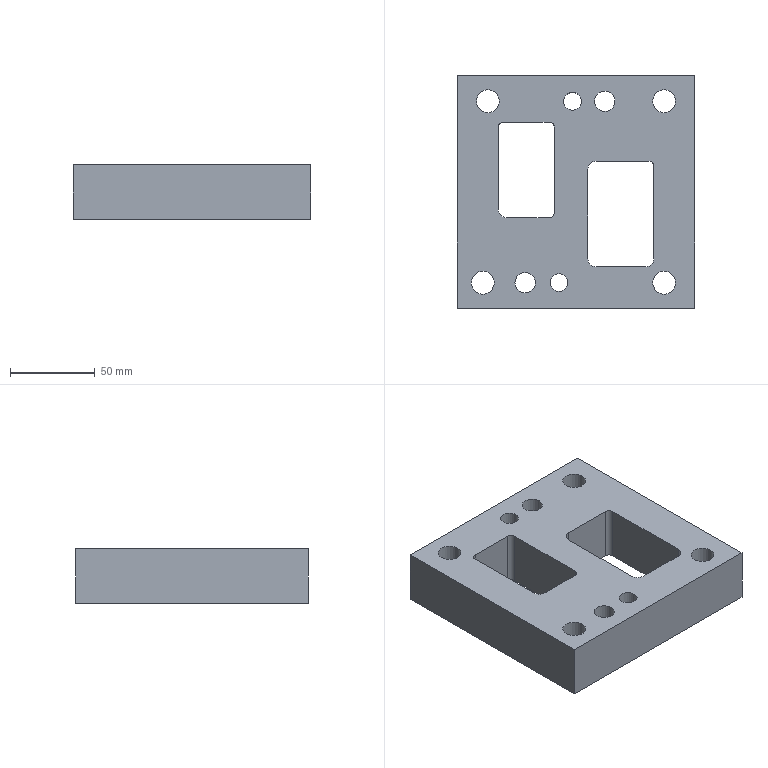Part | STEP file | lll_id3154_x_t | 1 solid | 38 faces | box 140 x 137 x 32 mm | volume 435633 mm3 | cylinder 20 | plane 18 | commonest cylinder face diameters 6 x4 10 x4 13.509 x4 20.008 x4 10.505 x2 12 x2
STEP:
#1=CARTESIAN_POINT('',(469.623,-270.25,60.5));
#2=VERTEX_POINT('',#1);
#3=CARTESIAN_POINT('',(464.37,-270.25,60.5));
#4=DIRECTION('',(0.,0.,1.));
#5=DIRECTION('',(1.,0.,0.));
#6=AXIS2_PLACEMENT_3D('',#3,#4,#5);
#7=CIRCLE('',#6,5.253);
#8=EDGE_CURVE('',#2,#2,#7,.T.);
#9=ORIENTED_EDGE('',*,*,#8,.T.);
#10=EDGE_LOOP('',(#9));
#11=FACE_BOUND('',#10,.T.);
#12=CARTESIAN_POINT('',(528.374,-377.25,60.5));
#13=VERTEX_POINT('',#12);
#14=CARTESIAN_POINT('',(518.37,-377.25,60.5));
#15=DIRECTION('',(0.,0.,-1.));
#16=DIRECTION('',(1.,0.,0.));
#17=AXIS2_PLACEMENT_3D('',#14,#15,#16);
#18=CIRCLE('',#17,10.004);
#19=EDGE_CURVE('',#13,#13,#18,.T.);
#20=ORIENTED_EDGE('',*,*,#19,.F.);
#21=EDGE_LOOP('',(#20));
#22=FACE_BOUND('',#21,.T.);
#23=CARTESIAN_POINT('',(442.371,-377.25,60.5));
#24=VERTEX_POINT('',#23);
#25=CARTESIAN_POINT('',(436.37,-377.25,60.5));
#26=DIRECTION('',(0.,0.,-1.));
#27=DIRECTION('',(1.,0.,0.));
#28=AXIS2_PLACEMENT_3D('',#25,#26,#27);
#29=CIRCLE('',#28,6.);
#30=EDGE_CURVE('',#24,#24,#29,.T.);
#31=ORIENTED_EDGE('',*,*,#30,.F.);
#32=EDGE_LOOP('',(#31));
#33=FACE_BOUND('',#32,.T.);
#34=CARTESIAN_POINT('',(528.374,-270.25,60.5));
#35=VERTEX_POINT('',#34);
#36=CARTESIAN_POINT('',(518.37,-270.25,60.5));
#37=DIRECTION('',(0.,0.,1.));
#38=DIRECTION('',(1.,0.,0.));
#39=AXIS2_PLACEMENT_3D('',#36,#37,#38);
#40=CIRCLE('',#39,10.004);
#41=EDGE_CURVE('',#35,#35,#40,.T.);
#42=ORIENTED_EDGE('',*,*,#41,.T.);
#43=EDGE_LOOP('',(#42));
#44=FACE_BOUND('',#43,.T.);
#45=CARTESIAN_POINT('',(507.37,-368.,60.5));
#46=VERTEX_POINT('',#45);
#47=CARTESIAN_POINT('',(478.37,-368.,60.5));
#48=VERTEX_POINT('',#47);
#49=CARTESIAN_POINT('',(492.87,-368.,60.5));
#50=DIRECTION('',(-1.,0.,0.));
#51=VECTOR('',#50,1.);
#52=LINE('',#49,#51);
#53=EDGE_CURVE('',#46,#48,#52,.T.);
#54=ORIENTED_EDGE('',*,*,#53,.F.);
#55=CARTESIAN_POINT('',(512.37,-363.,60.5));
#56=VERTEX_POINT('',#55);
#57=CARTESIAN_POINT('',(507.37,-363.,60.5));
#58=DIRECTION('',(0.,0.,1.));
#59=DIRECTION('',(-1.,0.,0.));
#60=AXIS2_PLACEMENT_3D('',#57,#58,#59);
#61=CIRCLE('',#60,5.);
#62=EDGE_CURVE('',#46,#56,#61,.T.);
#63=ORIENTED_EDGE('',*,*,#62,.T.);
#64=CARTESIAN_POINT('',(512.37,-308.5,60.5));
#65=VERTEX_POINT('',#64);
#66=CARTESIAN_POINT('',(512.37,-347.5,60.5));
#67=DIRECTION('',(0.,-1.,0.));
#68=VECTOR('',#67,1.);
#69=LINE('',#66,#68);
#70=EDGE_CURVE('',#65,#56,#69,.T.);
#71=ORIENTED_EDGE('',*,*,#70,.F.);
#72=CARTESIAN_POINT('',(509.37,-305.5,60.5));
#73=VERTEX_POINT('',#72);
#74=CARTESIAN_POINT('',(509.37,-308.5,60.5));
#75=DIRECTION('',(0.,0.,1.));
#76=DIRECTION('',(-1.,0.,0.));
#77=AXIS2_PLACEMENT_3D('',#74,#75,#76);
#78=CIRCLE('',#77,3.);
#79=EDGE_CURVE('',#65,#73,#78,.T.);
#80=ORIENTED_EDGE('',*,*,#79,.T.);
#81=CARTESIAN_POINT('',(478.37,-305.5,60.5));
#82=VERTEX_POINT('',#81);
#83=CARTESIAN_POINT('',(492.87,-305.5,60.5));
#84=DIRECTION('',(1.,0.,0.));
#85=VECTOR('',#84,1.);
#86=LINE('',#83,#85);
#87=EDGE_CURVE('',#82,#73,#86,.T.);
#88=ORIENTED_EDGE('',*,*,#87,.F.);
#89=CARTESIAN_POINT('',(473.37,-310.5,60.5));
#90=VERTEX_POINT('',#89);
#91=CARTESIAN_POINT('',(478.37,-310.5,60.5));
#92=DIRECTION('',(0.,0.,1.));
#93=DIRECTION('',(-1.,0.,0.));
#94=AXIS2_PLACEMENT_3D('',#91,#92,#93);
#95=CIRCLE('',#94,5.);
#96=EDGE_CURVE('',#82,#90,#95,.T.);
#97=ORIENTED_EDGE('',*,*,#96,.T.);
#98=CARTESIAN_POINT('',(473.37,-363.,60.5));
#99=VERTEX_POINT('',#98);
#100=CARTESIAN_POINT('',(473.37,-347.5,60.5));
#101=DIRECTION('',(0.,1.,0.));
#102=VECTOR('',#101,1.);
#103=LINE('',#100,#102);
#104=EDGE_CURVE('',#99,#90,#103,.T.);
#105=ORIENTED_EDGE('',*,*,#104,.F.);
#106=CARTESIAN_POINT('',(478.37,-363.,60.5));
#107=DIRECTION('',(0.,0.,1.));
#108=DIRECTION('',(-1.,0.,0.));
#109=AXIS2_PLACEMENT_3D('',#106,#107,#108);
#110=CIRCLE('',#109,5.);
#111=EDGE_CURVE('',#99,#48,#110,.T.);
#112=ORIENTED_EDGE('',*,*,#111,.T.);
#113=EDGE_LOOP('',(#54,#63,#71,#80,#88,#97,#105,#112));
#114=FACE_BOUND('',#113,.T.);
#115=CARTESIAN_POINT('',(536.37,-255.25,60.5));
#116=VERTEX_POINT('',#115);
#117=CARTESIAN_POINT('',(396.37,-255.25,60.5));
#118=VERTEX_POINT('',#117);
#119=CARTESIAN_POINT('',(466.37,-255.25,60.5));
#120=DIRECTION('',(-1.,0.,0.));
#121=VECTOR('',#120,1.);
#122=LINE('',#119,#121);
#123=EDGE_CURVE('',#116,#118,#122,.T.);
#124=ORIENTED_EDGE('',*,*,#123,.F.);
#125=CARTESIAN_POINT('',(536.37,-392.25,60.5));
#126=VERTEX_POINT('',#125);
#127=CARTESIAN_POINT('',(536.37,-325.25,60.5));
#128=DIRECTION('',(0.,1.,0.));
#129=VECTOR('',#128,1.);
#130=LINE('',#127,#129);
#131=EDGE_CURVE('',#126,#116,#130,.T.);
#132=ORIENTED_EDGE('',*,*,#131,.F.);
#133=CARTESIAN_POINT('',(396.37,-392.25,60.5));
#134=VERTEX_POINT('',#133);
#135=CARTESIAN_POINT('',(466.37,-392.25,60.5));
#136=DIRECTION('',(1.,0.,0.));
#137=VECTOR('',#136,1.);
#138=LINE('',#135,#137);
#139=EDGE_CURVE('',#134,#126,#138,.T.);
#140=ORIENTED_EDGE('',*,*,#139,.F.);
#141=CARTESIAN_POINT('',(396.37,-325.25,60.5));
#142=DIRECTION('',(0.,-1.,0.));
#143=VECTOR('',#142,1.);
#144=LINE('',#141,#143);
#145=EDGE_CURVE('',#118,#134,#144,.T.);
#146=ORIENTED_EDGE('',*,*,#145,.F.);
#147=EDGE_LOOP('',(#124,#132,#140,#146));
#148=FACE_BOUND('',#147,.T.);
#149=CARTESIAN_POINT('',(450.5,-282.5,60.5));
#150=VERTEX_POINT('',#149);
#151=CARTESIAN_POINT('',(423.5,-282.5,60.5));
#152=VERTEX_POINT('',#151);
#153=CARTESIAN_POINT('',(437.,-282.5,60.5));
#154=DIRECTION('',(-1.,0.,0.));
#155=VECTOR('',#154,1.);
#156=LINE('',#153,#155);
#157=EDGE_CURVE('',#150,#152,#156,.T.);
#158=ORIENTED_EDGE('',*,*,#157,.T.);
#159=CARTESIAN_POINT('',(420.5,-285.5,60.5));
#160=VERTEX_POINT('',#159);
#161=CARTESIAN_POINT('',(423.5,-285.5,60.5));
#162=DIRECTION('',(0.,0.,1.));
#163=DIRECTION('',(-1.,0.,0.));
#164=AXIS2_PLACEMENT_3D('',#161,#162,#163);
#165=CIRCLE('',#164,3.);
#166=EDGE_CURVE('',#152,#160,#165,.T.);
#167=ORIENTED_EDGE('',*,*,#166,.T.);
#168=CARTESIAN_POINT('',(420.5,-334.,60.5));
#169=VERTEX_POINT('',#168);
#170=CARTESIAN_POINT('',(420.5,-300.,60.5));
#171=DIRECTION('',(0.,-1.,0.));
#172=VECTOR('',#171,1.);
#173=LINE('',#170,#172);
#174=EDGE_CURVE('',#160,#169,#173,.T.);
#175=ORIENTED_EDGE('',*,*,#174,.T.);
#176=CARTESIAN_POINT('',(425.5,-339.,60.5));
#177=VERTEX_POINT('',#176);
#178=CARTESIAN_POINT('',(425.5,-334.,60.5));
#179=DIRECTION('',(0.,0.,1.));
#180=DIRECTION('',(-1.,0.,0.));
#181=AXIS2_PLACEMENT_3D('',#178,#179,#180);
#182=CIRCLE('',#181,5.);
#183=EDGE_CURVE('',#169,#177,#182,.T.);
#184=ORIENTED_EDGE('',*,*,#183,.T.);
#185=CARTESIAN_POINT('',(450.5,-339.,60.5));
#186=VERTEX_POINT('',#185);
#187=CARTESIAN_POINT('',(437.,-339.,60.5));
#188=DIRECTION('',(1.,0.,0.));
#189=VECTOR('',#188,1.);
#190=LINE('',#187,#189);
#191=EDGE_CURVE('',#177,#186,#190,.T.);
#192=ORIENTED_EDGE('',*,*,#191,.T.);
#193=CARTESIAN_POINT('',(453.5,-336.,60.5));
#194=VERTEX_POINT('',#193);
#195=CARTESIAN_POINT('',(450.5,-336.,60.5));
#196=DIRECTION('',(0.,0.,1.));
#197=DIRECTION('',(-1.,0.,0.));
#198=AXIS2_PLACEMENT_3D('',#195,#196,#197);
#199=CIRCLE('',#198,3.);
#200=EDGE_CURVE('',#186,#194,#199,.T.);
#201=ORIENTED_EDGE('',*,*,#200,.T.);
#202=CARTESIAN_POINT('',(453.5,-285.5,60.5));
#203=VERTEX_POINT('',#202);
#204=CARTESIAN_POINT('',(453.5,-300.,60.5));
#205=DIRECTION('',(0.,1.,0.));
#206=VECTOR('',#205,1.);
#207=LINE('',#204,#206);
#208=EDGE_CURVE('',#194,#203,#207,.T.);
#209=ORIENTED_EDGE('',*,*,#208,.T.);
#210=CARTESIAN_POINT('',(450.5,-285.5,60.5));
#211=DIRECTION('',(0.,0.,1.));
#212=DIRECTION('',(-1.,0.,0.));
#213=AXIS2_PLACEMENT_3D('',#210,#211,#212);
#214=CIRCLE('',#213,3.);
#215=EDGE_CURVE('',#203,#150,#214,.T.);
#216=ORIENTED_EDGE('',*,*,#215,.T.);
#217=EDGE_LOOP('',(#158,#167,#175,#184,#192,#201,#209,#216));
#218=FACE_BOUND('',#217,.T.);
#219=CARTESIAN_POINT('',(477.37,-270.25,60.5));
#220=VERTEX_POINT('',#219);
#221=CARTESIAN_POINT('',(483.37,-270.25,60.5));
#222=DIRECTION('',(0.,0.,-1.));
#223=DIRECTION('',(-1.,0.,0.));
#224=AXIS2_PLACEMENT_3D('',#221,#222,#223);
#225=CIRCLE('',#224,6.);
#226=EDGE_CURVE('',#220,#220,#225,.T.);
#227=ORIENTED_EDGE('',*,*,#226,.F.);
#228=EDGE_LOOP('',(#227));
#229=FACE_BOUND('',#228,.T.);
#230=CARTESIAN_POINT('',(404.366,-270.25,60.5));
#231=VERTEX_POINT('',#230);
#232=CARTESIAN_POINT('',(414.37,-270.25,60.5));
#233=DIRECTION('',(0.,0.,-1.));
#234=DIRECTION('',(-1.,0.,0.));
#235=AXIS2_PLACEMENT_3D('',#232,#233,#234);
#236=CIRCLE('',#235,10.004);
#237=EDGE_CURVE('',#231,#231,#236,.T.);
#238=ORIENTED_EDGE('',*,*,#237,.F.);
#239=EDGE_LOOP('',(#238));
#240=FACE_BOUND('',#239,.T.);
#241=CARTESIAN_POINT('',(401.366,-377.25,60.5));
#242=VERTEX_POINT('',#241);
#243=CARTESIAN_POINT('',(411.37,-377.25,60.5));
#244=DIRECTION('',(0.,0.,1.));
#245=DIRECTION('',(-1.,0.,0.));
#246=AXIS2_PLACEMENT_3D('',#243,#244,#245);
#247=CIRCLE('',#246,10.004);
#248=EDGE_CURVE('',#242,#242,#247,.T.);
#249=ORIENTED_EDGE('',*,*,#248,.T.);
#250=EDGE_LOOP('',(#249));
#251=FACE_BOUND('',#250,.T.);
#252=CARTESIAN_POINT('',(461.623,-377.25,60.5));
#253=VERTEX_POINT('',#252);
#254=CARTESIAN_POINT('',(456.37,-377.25,60.5));
#255=DIRECTION('',(0.,0.,1.));
#256=DIRECTION('',(1.,0.,0.));
#257=AXIS2_PLACEMENT_3D('',#254,#255,#256);
#258=CIRCLE('',#257,5.253);
#259=EDGE_CURVE('',#253,#253,#258,.T.);
#260=ORIENTED_EDGE('',*,*,#259,.T.);
#261=EDGE_LOOP('',(#260));
#262=FACE_BOUND('',#261,.T.);
#263=CARTESIAN_POINT('',(466.37,-325.25,60.5));
#264=DIRECTION('',(0.,0.,-1.));
#265=DIRECTION('',(0.,-1.,0.));
#266=AXIS2_PLACEMENT_3D('',#263,#264,#265);
#267=PLANE('',#266);
#268=ADVANCED_FACE('',(#11,#22,#33,#44,#114,#148,#218,#229,#240,#251,#262),#267,.T.);
#269=CARTESIAN_POINT('',(461.623,-377.25,92.5));
#270=VERTEX_POINT('',#269);
#271=CARTESIAN_POINT('',(456.37,-377.25,92.5));
#272=DIRECTION('',(0.,0.,1.));
#273=DIRECTION('',(1.,0.,0.));
#274=AXIS2_PLACEMENT_3D('',#271,#272,#273);
#275=CIRCLE('',#274,5.253);
#276=EDGE_CURVE('',#270,#270,#275,.T.);
#277=ORIENTED_EDGE('',*,*,#276,.F.);
#278=EDGE_LOOP('',(#277));
#279=FACE_BOUND('',#278,.T.);
#280=CARTESIAN_POINT('',(469.623,-270.25,92.5));
#281=VERTEX_POINT('',#280);
#282=CARTESIAN_POINT('',(464.37,-270.25,92.5));
#283=DIRECTION('',(0.,0.,1.));
#284=DIRECTION('',(1.,0.,0.));
#285=AXIS2_PLACEMENT_3D('',#282,#283,#284);
#286=CIRCLE('',#285,5.253);
#287=EDGE_CURVE('',#281,#281,#286,.T.);
#288=ORIENTED_EDGE('',*,*,#287,.F.);
#289=EDGE_LOOP('',(#288));
#290=FACE_BOUND('',#289,.T.);
#291=CARTESIAN_POINT('',(525.125,-377.25,92.5));
#292=VERTEX_POINT('',#291);
#293=CARTESIAN_POINT('',(518.37,-377.25,92.5));
#294=DIRECTION('',(0.,0.,1.));
#295=DIRECTION('',(1.,0.,0.));
#296=AXIS2_PLACEMENT_3D('',#293,#294,#295);
#297=CIRCLE('',#296,6.755);
#298=EDGE_CURVE('',#292,#292,#297,.T.);
#299=ORIENTED_EDGE('',*,*,#298,.F.);
#300=EDGE_LOOP('',(#299));
#301=FACE_BOUND('',#300,.T.);
#302=CARTESIAN_POINT('',(418.125,-377.25,92.5));
#303=VERTEX_POINT('',#302);
#304=CARTESIAN_POINT('',(411.37,-377.25,92.5));
#305=DIRECTION('',(0.,0.,1.));
#306=DIRECTION('',(1.,0.,0.));
#307=AXIS2_PLACEMENT_3D('',#304,#305,#306);
#308=CIRCLE('',#307,6.755);
#309=EDGE_CURVE('',#303,#303,#308,.T.);
#310=ORIENTED_EDGE('',*,*,#309,.F.);
#311=EDGE_LOOP('',(#310));
#312=FACE_BOUND('',#311,.T.);
#313=CARTESIAN_POINT('',(421.125,-270.25,92.5));
#314=VERTEX_POINT('',#313);
#315=CARTESIAN_POINT('',(414.37,-270.25,92.5));
#316=DIRECTION('',(0.,0.,1.));
#317=DIRECTION('',(1.,0.,0.));
#318=AXIS2_PLACEMENT_3D('',#315,#316,#317);
#319=CIRCLE('',#318,6.755);
#320=EDGE_CURVE('',#314,#314,#319,.T.);
#321=ORIENTED_EDGE('',*,*,#320,.F.);
#322=EDGE_LOOP('',(#321));
#323=FACE_BOUND('',#322,.T.);
#324=CARTESIAN_POINT('',(525.125,-270.25,92.5));
#325=VERTEX_POINT('',#324);
#326=CARTESIAN_POINT('',(518.37,-270.25,92.5));
#327=DIRECTION('',(0.,0.,1.));
#328=DIRECTION('',(1.,0.,0.));
#329=AXIS2_PLACEMENT_3D('',#326,#327,#328);
#330=CIRCLE('',#329,6.755);
#331=EDGE_CURVE('',#325,#325,#330,.T.);
#332=ORIENTED_EDGE('',*,*,#331,.F.);
#333=EDGE_LOOP('',(#332));
#334=FACE_BOUND('',#333,.T.);
#335=CARTESIAN_POINT('',(536.37,-255.25,92.5));
#336=VERTEX_POINT('',#335);
#337=CARTESIAN_POINT('',(536.37,-392.25,92.5));
#338=VERTEX_POINT('',#337);
#339=CARTESIAN_POINT('',(536.37,-325.25,92.5));
#340=DIRECTION('',(0.,-1.,0.));
#341=VECTOR('',#340,1.);
#342=LINE('',#339,#341);
#343=EDGE_CURVE('',#336,#338,#342,.T.);
#344=ORIENTED_EDGE('',*,*,#343,.F.);
#345=CARTESIAN_POINT('',(396.37,-255.25,92.5));
#346=VERTEX_POINT('',#345);
#347=CARTESIAN_POINT('',(466.37,-255.25,92.5));
#348=DIRECTION('',(1.,0.,0.));
#349=VECTOR('',#348,1.);
#350=LINE('',#347,#349);
#351=EDGE_CURVE('',#346,#336,#350,.T.);
#352=ORIENTED_EDGE('',*,*,#351,.F.);
#353=CARTESIAN_POINT('',(396.37,-392.25,92.5));
#354=VERTEX_POINT('',#353);
#355=CARTESIAN_POINT('',(396.37,-325.25,92.5));
#356=DIRECTION('',(0.,1.,0.));
#357=VECTOR('',#356,1.);
#358=LINE('',#355,#357);
#359=EDGE_CURVE('',#354,#346,#358,.T.);
#360=ORIENTED_EDGE('',*,*,#359,.F.);
#361=CARTESIAN_POINT('',(466.37,-392.25,92.5));
#362=DIRECTION('',(-1.,0.,0.));
#363=VECTOR('',#362,1.);
#364=LINE('',#361,#363);
#365=EDGE_CURVE('',#338,#354,#364,.T.);
#366=ORIENTED_EDGE('',*,*,#365,.F.);
#367=EDGE_LOOP('',(#344,#352,#360,#366));
#368=FACE_BOUND('',#367,.T.);
#369=CARTESIAN_POINT('',(509.37,-305.5,92.5));
#370=VERTEX_POINT('',#369);
#371=CARTESIAN_POINT('',(478.37,-305.5,92.5));
#372=VERTEX_POINT('',#371);
#373=CARTESIAN_POINT('',(492.87,-305.5,92.5));
#374=DIRECTION('',(-1.,0.,0.));
#375=VECTOR('',#374,1.);
#376=LINE('',#373,#375);
#377=EDGE_CURVE('',#370,#372,#376,.T.);
#378=ORIENTED_EDGE('',*,*,#377,.F.);
#379=CARTESIAN_POINT('',(512.37,-308.5,92.5));
#380=VERTEX_POINT('',#379);
#381=CARTESIAN_POINT('',(509.37,-308.5,92.5));
#382=DIRECTION('',(0.,0.,-1.));
#383=DIRECTION('',(1.,0.,0.));
#384=AXIS2_PLACEMENT_3D('',#381,#382,#383);
#385=CIRCLE('',#384,3.);
#386=EDGE_CURVE('',#370,#380,#385,.T.);
#387=ORIENTED_EDGE('',*,*,#386,.T.);
#388=CARTESIAN_POINT('',(512.37,-363.,92.5));
#389=VERTEX_POINT('',#388);
#390=CARTESIAN_POINT('',(512.37,-347.5,92.5));
#391=DIRECTION('',(0.,1.,0.));
#392=VECTOR('',#391,1.);
#393=LINE('',#390,#392);
#394=EDGE_CURVE('',#389,#380,#393,.T.);
#395=ORIENTED_EDGE('',*,*,#394,.F.);
#396=CARTESIAN_POINT('',(507.37,-368.,92.5));
#397=VERTEX_POINT('',#396);
#398=CARTESIAN_POINT('',(507.37,-363.,92.5));
#399=DIRECTION('',(0.,0.,-1.));
#400=DIRECTION('',(1.,0.,0.));
#401=AXIS2_PLACEMENT_3D('',#398,#399,#400);
#402=CIRCLE('',#401,5.);
#403=EDGE_CURVE('',#389,#397,#402,.T.);
#404=ORIENTED_EDGE('',*,*,#403,.T.);
#405=CARTESIAN_POINT('',(478.37,-368.,92.5));
#406=VERTEX_POINT('',#405);
#407=CARTESIAN_POINT('',(492.87,-368.,92.5));
#408=DIRECTION('',(1.,0.,0.));
#409=VECTOR('',#408,1.);
#410=LINE('',#407,#409);
#411=EDGE_CURVE('',#406,#397,#410,.T.);
#412=ORIENTED_EDGE('',*,*,#411,.F.);
#413=CARTESIAN_POINT('',(473.37,-363.,92.5));
#414=VERTEX_POINT('',#413);
#415=CARTESIAN_POINT('',(478.37,-363.,92.5));
#416=DIRECTION('',(0.,0.,-1.));
#417=DIRECTION('',(1.,0.,0.));
#418=AXIS2_PLACEMENT_3D('',#415,#416,#417);
#419=CIRCLE('',#418,5.);
#420=EDGE_CURVE('',#406,#414,#419,.T.);
#421=ORIENTED_EDGE('',*,*,#420,.T.);
#422=CARTESIAN_POINT('',(473.37,-310.5,92.5));
#423=VERTEX_POINT('',#422);
#424=CARTESIAN_POINT('',(473.37,-347.5,92.5));
#425=DIRECTION('',(0.,-1.,0.));
#426=VECTOR('',#425,1.);
#427=LINE('',#424,#426);
#428=EDGE_CURVE('',#423,#414,#427,.T.);
#429=ORIENTED_EDGE('',*,*,#428,.F.);
#430=CARTESIAN_POINT('',(478.37,-310.5,92.5));
#431=DIRECTION('',(0.,0.,-1.));
#432=DIRECTION('',(1.,0.,0.));
#433=AXIS2_PLACEMENT_3D('',#430,#431,#432);
#434=CIRCLE('',#433,5.);
#435=EDGE_CURVE('',#423,#372,#434,.T.);
#436=ORIENTED_EDGE('',*,*,#435,.T.);
#437=EDGE_LOOP('',(#378,#387,#395,#404,#412,#421,#429,#436));
#438=FACE_BOUND('',#437,.T.);
#439=CARTESIAN_POINT('',(420.5,-334.,92.5));
#440=VERTEX_POINT('',#439);
#441=CARTESIAN_POINT('',(420.5,-285.5,92.5));
#442=VERTEX_POINT('',#441);
#443=CARTESIAN_POINT('',(420.5,-300.,92.5));
#444=DIRECTION('',(0.,1.,0.));
#445=VECTOR('',#444,1.);
#446=LINE('',#443,#445);
#447=EDGE_CURVE('',#440,#442,#446,.T.);
#448=ORIENTED_EDGE('',*,*,#447,.T.);
#449=CARTESIAN_POINT('',(423.5,-282.5,92.5));
#450=VERTEX_POINT('',#449);
#451=CARTESIAN_POINT('',(423.5,-285.5,92.5));
#452=DIRECTION('',(0.,0.,-1.));
#453=DIRECTION('',(1.,0.,0.));
#454=AXIS2_PLACEMENT_3D('',#451,#452,#453);
#455=CIRCLE('',#454,3.);
#456=EDGE_CURVE('',#442,#450,#455,.T.);
#457=ORIENTED_EDGE('',*,*,#456,.T.);
#458=CARTESIAN_POINT('',(450.5,-282.5,92.5));
#459=VERTEX_POINT('',#458);
#460=CARTESIAN_POINT('',(437.,-282.5,92.5));
#461=DIRECTION('',(1.,0.,0.));
#462=VECTOR('',#461,1.);
#463=LINE('',#460,#462);
#464=EDGE_CURVE('',#450,#459,#463,.T.);
#465=ORIENTED_EDGE('',*,*,#464,.T.);
#466=CARTESIAN_POINT('',(453.5,-285.5,92.5));
#467=VERTEX_POINT('',#466);
#468=CARTESIAN_POINT('',(450.5,-285.5,92.5));
#469=DIRECTION('',(0.,0.,-1.));
#470=DIRECTION('',(1.,0.,0.));
#471=AXIS2_PLACEMENT_3D('',#468,#469,#470);
#472=CIRCLE('',#471,3.);
#473=EDGE_CURVE('',#459,#467,#472,.T.);
#474=ORIENTED_EDGE('',*,*,#473,.T.);
#475=CARTESIAN_POINT('',(453.5,-336.,92.5));
#476=VERTEX_POINT('',#475);
#477=CARTESIAN_POINT('',(453.5,-300.,92.5));
#478=DIRECTION('',(0.,-1.,0.));
#479=VECTOR('',#478,1.);
#480=LINE('',#477,#479);
#481=EDGE_CURVE('',#467,#476,#480,.T.);
#482=ORIENTED_EDGE('',*,*,#481,.T.);
#483=CARTESIAN_POINT('',(450.5,-339.,92.5));
#484=VERTEX_POINT('',#483);
#485=CARTESIAN_POINT('',(450.5,-336.,92.5));
#486=DIRECTION('',(0.,0.,-1.));
#487=DIRECTION('',(1.,0.,0.));
#488=AXIS2_PLACEMENT_3D('',#485,#486,#487);
#489=CIRCLE('',#488,3.);
#490=EDGE_CURVE('',#476,#484,#489,.T.);
#491=ORIENTED_EDGE('',*,*,#490,.T.);
#492=CARTESIAN_POINT('',(425.5,-339.,92.5));
#493=VERTEX_POINT('',#492);
#494=CARTESIAN_POINT('',(437.,-339.,92.5));
#495=DIRECTION('',(-1.,0.,0.));
#496=VECTOR('',#495,1.);
#497=LINE('',#494,#496);
#498=EDGE_CURVE('',#484,#493,#497,.T.);
#499=ORIENTED_EDGE('',*,*,#498,.T.);
#500=CARTESIAN_POINT('',(425.5,-334.,92.5));
#501=DIRECTION('',(0.,0.,-1.));
#502=DIRECTION('',(1.,0.,0.));
#503=AXIS2_PLACEMENT_3D('',#500,#501,#502);
#504=CIRCLE('',#503,5.);
#505=EDGE_CURVE('',#493,#440,#504,.T.);
#506=ORIENTED_EDGE('',*,*,#505,.T.);
#507=EDGE_LOOP('',(#448,#457,#465,#474,#482,#491,#499,#506));
#508=FACE_BOUND('',#507,.T.);
#509=CARTESIAN_POINT('',(489.371,-270.25,92.5));
#510=VERTEX_POINT('',#509);
#511=CARTESIAN_POINT('',(483.37,-270.25,92.5));
#512=DIRECTION('',(0.,0.,-1.));
#513=DIRECTION('',(1.,0.,0.));
#514=AXIS2_PLACEMENT_3D('',#511,#512,#513);
#515=CIRCLE('',#514,6.);
#516=EDGE_CURVE('',#510,#510,#515,.T.);
#517=ORIENTED_EDGE('',*,*,#516,.T.);
#518=EDGE_LOOP('',(#517));
#519=FACE_BOUND('',#518,.T.);
#520=CARTESIAN_POINT('',(430.37,-377.25,92.5));
#521=VERTEX_POINT('',#520);
#522=CARTESIAN_POINT('',(436.37,-377.25,92.5));
#523=DIRECTION('',(0.,0.,-1.));
#524=DIRECTION('',(-1.,0.,0.));
#525=AXIS2_PLACEMENT_3D('',#522,#523,#524);
#526=CIRCLE('',#525,6.);
#527=EDGE_CURVE('',#521,#521,#526,.T.);
#528=ORIENTED_EDGE('',*,*,#527,.T.);
#529=EDGE_LOOP('',(#528));
#530=FACE_BOUND('',#529,.T.);
#531=CARTESIAN_POINT('',(466.37,-325.25,92.5));
#532=DIRECTION('',(0.,0.,1.));
#533=DIRECTION('',(0.,1.,0.));
#534=AXIS2_PLACEMENT_3D('',#531,#532,#533);
#535=PLANE('',#534);
#536=ADVANCED_FACE('',(#279,#290,#301,#312,#323,#334,#368,#438,#508,#519,#530),#535,.T.);
#537=CARTESIAN_POINT('',(536.37,-255.25,60.5));
#538=DIRECTION('',(0.,0.,1.));
#539=VECTOR('',#538,1.);
#540=LINE('',#537,#539);
#541=EDGE_CURVE('',#116,#336,#540,.T.);
#542=ORIENTED_EDGE('',*,*,#541,.T.);
#543=ORIENTED_EDGE('',*,*,#343,.T.);
#544=CARTESIAN_POINT('',(536.37,-392.25,60.5));
#545=DIRECTION('',(0.,0.,1.));
#546=VECTOR('',#545,1.);
#547=LINE('',#544,#546);
#548=EDGE_CURVE('',#126,#338,#547,.T.);
#549=ORIENTED_EDGE('',*,*,#548,.F.);
#550=ORIENTED_EDGE('',*,*,#131,.T.);
#551=EDGE_LOOP('',(#542,#543,#549,#550));
#552=FACE_OUTER_BOUND('',#551,.T.);
#553=CARTESIAN_POINT('',(536.37,-325.25,60.5));
#554=DIRECTION('',(1.,0.,0.));
#555=DIRECTION('',(0.,0.,-1.));
#556=AXIS2_PLACEMENT_3D('',#553,#554,#555);
#557=PLANE('',#556);
#558=ADVANCED_FACE('',(#552),#557,.T.);
#559=ORIENTED_EDGE('',*,*,#548,.T.);
#560=ORIENTED_EDGE('',*,*,#365,.T.);
#561=CARTESIAN_POINT('',(396.37,-392.25,60.5));
#562=DIRECTION('',(0.,0.,1.));
#563=VECTOR('',#562,1.);
#564=LINE('',#561,#563);
#565=EDGE_CURVE('',#134,#354,#564,.T.);
#566=ORIENTED_EDGE('',*,*,#565,.F.);
#567=ORIENTED_EDGE('',*,*,#139,.T.);
#568=EDGE_LOOP('',(#559,#560,#566,#567));
#569=FACE_OUTER_BOUND('',#568,.T.);
#570=CARTESIAN_POINT('',(466.37,-392.25,60.5));
#571=DIRECTION('',(0.,-1.,0.));
#572=DIRECTION('',(0.,0.,1.));
#573=AXIS2_PLACEMENT_3D('',#570,#571,#572);
#574=PLANE('',#573);
#575=ADVANCED_FACE('',(#569),#574,.T.);
#576=ORIENTED_EDGE('',*,*,#565,.T.);
#577=ORIENTED_EDGE('',*,*,#359,.T.);
#578=CARTESIAN_POINT('',(396.37,-255.25,60.5));
#579=DIRECTION('',(0.,0.,1.));
#580=VECTOR('',#579,1.);
#581=LINE('',#578,#580);
#582=EDGE_CURVE('',#118,#346,#581,.T.);
#583=ORIENTED_EDGE('',*,*,#582,.F.);
#584=ORIENTED_EDGE('',*,*,#145,.T.);
#585=EDGE_LOOP('',(#576,#577,#583,#584));
#586=FACE_OUTER_BOUND('',#585,.T.);
#587=CARTESIAN_POINT('',(396.37,-325.25,60.5));
#588=DIRECTION('',(-1.,0.,0.));
#589=DIRECTION('',(0.,0.,1.));
#590=AXIS2_PLACEMENT_3D('',#587,#588,#589);
#591=PLANE('',#590);
#592=ADVANCED_FACE('',(#586),#591,.T.);
#593=ORIENTED_EDGE('',*,*,#123,.T.);
#594=ORIENTED_EDGE('',*,*,#582,.T.);
#595=ORIENTED_EDGE('',*,*,#351,.T.);
#596=ORIENTED_EDGE('',*,*,#541,.F.);
#597=EDGE_LOOP('',(#593,#594,#595,#596));
#598=FACE_OUTER_BOUND('',#597,.T.);
#599=CARTESIAN_POINT('',(466.37,-255.25,60.5));
#600=DIRECTION('',(0.,1.,0.));
#601=DIRECTION('',(0.,0.,-1.));
#602=AXIS2_PLACEMENT_3D('',#599,#600,#601);
#603=PLANE('',#602);
#604=ADVANCED_FACE('',(#598),#603,.T.);
#605=ORIENTED_EDGE('',*,*,#411,.T.);
#606=CARTESIAN_POINT('',(507.37,-368.,60.5));
#607=DIRECTION('',(0.,0.,-1.));
#608=VECTOR('',#607,1.);
#609=LINE('',#606,#608);
#610=EDGE_CURVE('',#397,#46,#609,.T.);
#611=ORIENTED_EDGE('',*,*,#610,.T.);
#612=ORIENTED_EDGE('',*,*,#53,.T.);
#613=CARTESIAN_POINT('',(478.37,-368.,92.5));
#614=DIRECTION('',(0.,0.,1.));
#615=VECTOR('',#614,1.);
#616=LINE('',#613,#615);
#617=EDGE_CURVE('',#48,#406,#616,.T.);
#618=ORIENTED_EDGE('',*,*,#617,.T.);
#619=EDGE_LOOP('',(#605,#611,#612,#618));
#620=FACE_OUTER_BOUND('',#619,.T.);
#621=CARTESIAN_POINT('',(492.87,-368.,-8.5));
#622=DIRECTION('',(0.,-1.,0.));
#623=DIRECTION('',(0.,0.,-1.));
#624=AXIS2_PLACEMENT_3D('',#621,#622,#623);
#625=PLANE('',#624);
#626=ADVANCED_FACE('',(#620),#625,.F.);
#627=ORIENTED_EDGE('',*,*,#104,.T.);
#628=CARTESIAN_POINT('',(473.37,-310.5,92.5));
#629=DIRECTION('',(0.,0.,1.));
#630=VECTOR('',#629,1.);
#631=LINE('',#628,#630);
#632=EDGE_CURVE('',#90,#423,#631,.T.);
#633=ORIENTED_EDGE('',*,*,#632,.T.);
#634=ORIENTED_EDGE('',*,*,#428,.T.);
#635=CARTESIAN_POINT('',(473.37,-363.,60.5));
#636=DIRECTION('',(0.,0.,-1.));
#637=VECTOR('',#636,1.);
#638=LINE('',#635,#637);
#639=EDGE_CURVE('',#414,#99,#638,.T.);
#640=ORIENTED_EDGE('',*,*,#639,.T.);
#641=EDGE_LOOP('',(#627,#633,#634,#640));
#642=FACE_OUTER_BOUND('',#641,.T.);
#643=CARTESIAN_POINT('',(473.37,-347.5,-8.5));
#644=DIRECTION('',(-1.,0.,0.));
#645=DIRECTION('',(0.,0.,-1.));
#646=AXIS2_PLACEMENT_3D('',#643,#644,#645);
#647=PLANE('',#646);
#648=ADVANCED_FACE('',(#642),#647,.F.);
#649=ORIENTED_EDGE('',*,*,#87,.T.);
#650=CARTESIAN_POINT('',(509.37,-305.5,92.5));
#651=DIRECTION('',(0.,0.,1.));
#652=VECTOR('',#651,1.);
#653=LINE('',#650,#652);
#654=EDGE_CURVE('',#73,#370,#653,.T.);
#655=ORIENTED_EDGE('',*,*,#654,.T.);
#656=ORIENTED_EDGE('',*,*,#377,.T.);
#657=CARTESIAN_POINT('',(478.37,-305.5,60.5));
#658=DIRECTION('',(0.,0.,-1.));
#659=VECTOR('',#658,1.);
#660=LINE('',#657,#659);
#661=EDGE_CURVE('',#372,#82,#660,.T.);
#662=ORIENTED_EDGE('',*,*,#661,.T.);
#663=EDGE_LOOP('',(#649,#655,#656,#662));
#664=FACE_OUTER_BOUND('',#663,.T.);
#665=CARTESIAN_POINT('',(492.87,-305.5,-8.5));
#666=DIRECTION('',(0.,1.,0.));
#667=DIRECTION('',(0.,0.,1.));
#668=AXIS2_PLACEMENT_3D('',#665,#666,#667);
#669=PLANE('',#668);
#670=ADVANCED_FACE('',(#664),#669,.F.);
#671=ORIENTED_EDGE('',*,*,#394,.T.);
#672=CARTESIAN_POINT('',(512.37,-308.5,60.5));
#673=DIRECTION('',(0.,0.,-1.));
#674=VECTOR('',#673,1.);
#675=LINE('',#672,#674);
#676=EDGE_CURVE('',#380,#65,#675,.T.);
#677=ORIENTED_EDGE('',*,*,#676,.T.);
#678=ORIENTED_EDGE('',*,*,#70,.T.);
#679=CARTESIAN_POINT('',(512.37,-363.,92.5));
#680=DIRECTION('',(0.,0.,1.));
#681=VECTOR('',#680,1.);
#682=LINE('',#679,#681);
#683=EDGE_CURVE('',#56,#389,#682,.T.);
#684=ORIENTED_EDGE('',*,*,#683,.T.);
#685=EDGE_LOOP('',(#671,#677,#678,#684));
#686=FACE_OUTER_BOUND('',#685,.T.);
#687=CARTESIAN_POINT('',(512.37,-347.5,-8.5));
#688=DIRECTION('',(1.,0.,0.));
#689=DIRECTION('',(0.,0.,1.));
#690=AXIS2_PLACEMENT_3D('',#687,#688,#689);
#691=PLANE('',#690);
#692=ADVANCED_FACE('',(#686),#691,.F.);
#693=ORIENTED_EDGE('',*,*,#498,.F.);
#694=CARTESIAN_POINT('',(450.5,-339.,60.5));
#695=DIRECTION('',(0.,0.,-1.));
#696=VECTOR('',#695,1.);
#697=LINE('',#694,#696);
#698=EDGE_CURVE('',#484,#186,#697,.T.);
#699=ORIENTED_EDGE('',*,*,#698,.T.);
#700=ORIENTED_EDGE('',*,*,#191,.F.);
#701=CARTESIAN_POINT('',(425.5,-339.,92.5));
#702=DIRECTION('',(0.,0.,1.));
#703=VECTOR('',#702,1.);
#704=LINE('',#701,#703);
#705=EDGE_CURVE('',#177,#493,#704,.T.);
#706=ORIENTED_EDGE('',*,*,#705,.T.);
#707=EDGE_LOOP('',(#693,#699,#700,#706));
#708=FACE_OUTER_BOUND('',#707,.T.);
#709=CARTESIAN_POINT('',(437.,-339.,-8.5));
#710=DIRECTION('',(0.,-1.,0.));
#711=DIRECTION('',(0.,0.,1.));
#712=AXIS2_PLACEMENT_3D('',#709,#710,#711);
#713=PLANE('',#712);
#714=ADVANCED_FACE('',(#708),#713,.F.);
#715=ORIENTED_EDGE('',*,*,#174,.F.);
#716=CARTESIAN_POINT('',(420.5,-285.5,92.5));
#717=DIRECTION('',(0.,0.,1.));
#718=VECTOR('',#717,1.);
#719=LINE('',#716,#718);
#720=EDGE_CURVE('',#160,#442,#719,.T.);
#721=ORIENTED_EDGE('',*,*,#720,.T.);
#722=ORIENTED_EDGE('',*,*,#447,.F.);
#723=CARTESIAN_POINT('',(420.5,-334.,60.5));
#724=DIRECTION('',(0.,0.,-1.));
#725=VECTOR('',#724,1.);
#726=LINE('',#723,#725);
#727=EDGE_CURVE('',#440,#169,#726,.T.);
#728=ORIENTED_EDGE('',*,*,#727,.T.);
#729=EDGE_LOOP('',(#715,#721,#722,#728));
#730=FACE_OUTER_BOUND('',#729,.T.);
#731=CARTESIAN_POINT('',(420.5,-300.,-8.5));
#732=DIRECTION('',(-1.,0.,0.));
#733=DIRECTION('',(0.,0.,-1.));
#734=AXIS2_PLACEMENT_3D('',#731,#732,#733);
#735=PLANE('',#734);
#736=ADVANCED_FACE('',(#730),#735,.F.);
#737=ORIENTED_EDGE('',*,*,#464,.F.);
#738=CARTESIAN_POINT('',(423.5,-282.5,60.5));
#739=DIRECTION('',(0.,0.,-1.));
#740=VECTOR('',#739,1.);
#741=LINE('',#738,#740);
#742=EDGE_CURVE('',#450,#152,#741,.T.);
#743=ORIENTED_EDGE('',*,*,#742,.T.);
#744=ORIENTED_EDGE('',*,*,#157,.F.);
#745=CARTESIAN_POINT('',(450.5,-282.5,92.5));
#746=DIRECTION('',(0.,0.,1.));
#747=VECTOR('',#746,1.);
#748=LINE('',#745,#747);
#749=EDGE_CURVE('',#150,#459,#748,.T.);
#750=ORIENTED_EDGE('',*,*,#749,.T.);
#751=EDGE_LOOP('',(#737,#743,#744,#750));
#752=FACE_OUTER_BOUND('',#751,.T.);
#753=CARTESIAN_POINT('',(437.,-282.5,-8.5));
#754=DIRECTION('',(0.,1.,0.));
#755=DIRECTION('',(0.,0.,-1.));
#756=AXIS2_PLACEMENT_3D('',#753,#754,#755);
#757=PLANE('',#756);
#758=ADVANCED_FACE('',(#752),#757,.F.);
#759=ORIENTED_EDGE('',*,*,#208,.F.);
#760=CARTESIAN_POINT('',(453.5,-336.,92.5));
#761=DIRECTION('',(0.,0.,1.));
#762=VECTOR('',#761,1.);
#763=LINE('',#760,#762);
#764=EDGE_CURVE('',#194,#476,#763,.T.);
#765=ORIENTED_EDGE('',*,*,#764,.T.);
#766=ORIENTED_EDGE('',*,*,#481,.F.);
#767=CARTESIAN_POINT('',(453.5,-285.5,60.5));
#768=DIRECTION('',(0.,0.,-1.));
#769=VECTOR('',#768,1.);
#770=LINE('',#767,#769);
#771=EDGE_CURVE('',#467,#203,#770,.T.);
#772=ORIENTED_EDGE('',*,*,#771,.T.);
#773=EDGE_LOOP('',(#759,#765,#766,#772));
#774=FACE_OUTER_BOUND('',#773,.T.);
#775=CARTESIAN_POINT('',(453.5,-300.,-8.5));
#776=DIRECTION('',(1.,0.,0.));
#777=DIRECTION('',(0.,0.,1.));
#778=AXIS2_PLACEMENT_3D('',#775,#776,#777);
#779=PLANE('',#778);
#780=ADVANCED_FACE('',(#774),#779,.F.);
#781=CARTESIAN_POINT('',(528.374,-270.25,75.5));
#782=VERTEX_POINT('',#781);
#783=CARTESIAN_POINT('',(518.37,-270.25,75.5));
#784=DIRECTION('',(0.,0.,1.));
#785=DIRECTION('',(1.,0.,0.));
#786=AXIS2_PLACEMENT_3D('',#783,#784,#785);
#787=CIRCLE('',#786,10.004);
#788=EDGE_CURVE('',#782,#782,#787,.T.);
#789=ORIENTED_EDGE('',*,*,#788,.T.);
#790=EDGE_LOOP('',(#789));
#791=FACE_BOUND('',#790,.T.);
#792=ORIENTED_EDGE('',*,*,#41,.F.);
#793=EDGE_LOOP('',(#792));
#794=FACE_BOUND('',#793,.T.);
#795=CARTESIAN_POINT('',(518.37,-270.25,60.5));
#796=DIRECTION('',(0.,0.,1.));
#797=DIRECTION('',(1.,0.,0.));
#798=AXIS2_PLACEMENT_3D('',#795,#796,#797);
#799=CYLINDRICAL_SURFACE('',#798,10.004);
#800=ADVANCED_FACE('',(#791,#794),#799,.F.);
#801=ORIENTED_EDGE('',*,*,#331,.T.);
#802=EDGE_LOOP('',(#801));
#803=FACE_BOUND('',#802,.T.);
#804=CARTESIAN_POINT('',(525.125,-270.25,75.5));
#805=VERTEX_POINT('',#804);
#806=CARTESIAN_POINT('',(518.37,-270.25,75.5));
#807=DIRECTION('',(0.,0.,1.));
#808=DIRECTION('',(1.,0.,0.));
#809=AXIS2_PLACEMENT_3D('',#806,#807,#808);
#810=CIRCLE('',#809,6.755);
#811=EDGE_CURVE('',#805,#805,#810,.T.);
#812=ORIENTED_EDGE('',*,*,#811,.F.);
#813=EDGE_LOOP('',(#812));
#814=FACE_BOUND('',#813,.T.);
#815=CARTESIAN_POINT('',(518.37,-270.25,57.5));
#816=DIRECTION('',(0.,0.,1.));
#817=DIRECTION('',(1.,0.,0.));
#818=AXIS2_PLACEMENT_3D('',#815,#816,#817);
#819=CYLINDRICAL_SURFACE('',#818,6.755);
#820=ADVANCED_FACE('',(#803,#814),#819,.F.);
#821=ORIENTED_EDGE('',*,*,#811,.T.);
#822=EDGE_LOOP('',(#821));
#823=FACE_BOUND('',#822,.T.);
#824=ORIENTED_EDGE('',*,*,#788,.F.);
#825=EDGE_LOOP('',(#824));
#826=FACE_BOUND('',#825,.T.);
#827=CARTESIAN_POINT('',(518.37,-270.25,75.5));
#828=DIRECTION('',(0.,0.,1.));
#829=DIRECTION('',(1.,0.,0.));
#830=AXIS2_PLACEMENT_3D('',#827,#828,#829);
#831=PLANE('',#830);
#832=ADVANCED_FACE('',(#823,#826),#831,.F.);
#833=ORIENTED_EDGE('',*,*,#226,.T.);
#834=EDGE_LOOP('',(#833));
#835=FACE_BOUND('',#834,.T.);
#836=ORIENTED_EDGE('',*,*,#516,.F.);
#837=EDGE_LOOP('',(#836));
#838=FACE_BOUND('',#837,.T.);
#839=CARTESIAN_POINT('',(483.37,-270.25,57.5));
#840=DIRECTION('',(0.,0.,1.));
#841=DIRECTION('',(1.,0.,0.));
#842=AXIS2_PLACEMENT_3D('',#839,#840,#841);
#843=CYLINDRICAL_SURFACE('',#842,6.);
#844=ADVANCED_FACE('',(#835,#838),#843,.F.);
#845=CARTESIAN_POINT('',(404.366,-270.25,75.5));
#846=VERTEX_POINT('',#845);
#847=CARTESIAN_POINT('',(414.37,-270.25,75.5));
#848=DIRECTION('',(0.,0.,-1.));
#849=DIRECTION('',(-1.,0.,0.));
#850=AXIS2_PLACEMENT_3D('',#847,#848,#849);
#851=CIRCLE('',#850,10.004);
#852=EDGE_CURVE('',#846,#846,#851,.T.);
#853=ORIENTED_EDGE('',*,*,#852,.F.);
#854=EDGE_LOOP('',(#853));
#855=FACE_BOUND('',#854,.T.);
#856=ORIENTED_EDGE('',*,*,#237,.T.);
#857=EDGE_LOOP('',(#856));
#858=FACE_BOUND('',#857,.T.);
#859=CARTESIAN_POINT('',(414.37,-270.25,60.5));
#860=DIRECTION('',(0.,0.,1.));
#861=DIRECTION('',(-1.,0.,0.));
#862=AXIS2_PLACEMENT_3D('',#859,#860,#861);
#863=CYLINDRICAL_SURFACE('',#862,10.004);
#864=ADVANCED_FACE('',(#855,#858),#863,.F.);
#865=ORIENTED_EDGE('',*,*,#320,.T.);
#866=EDGE_LOOP('',(#865));
#867=FACE_BOUND('',#866,.T.);
#868=CARTESIAN_POINT('',(407.616,-270.25,75.5));
#869=VERTEX_POINT('',#868);
#870=CARTESIAN_POINT('',(414.37,-270.25,75.5));
#871=DIRECTION('',(0.,0.,-1.));
#872=DIRECTION('',(-1.,0.,0.));
#873=AXIS2_PLACEMENT_3D('',#870,#871,#872);
#874=CIRCLE('',#873,6.755);
#875=EDGE_CURVE('',#869,#869,#874,.T.);
#876=ORIENTED_EDGE('',*,*,#875,.T.);
#877=EDGE_LOOP('',(#876));
#878=FACE_BOUND('',#877,.T.);
#879=CARTESIAN_POINT('',(414.37,-270.25,57.5));
#880=DIRECTION('',(0.,0.,1.));
#881=DIRECTION('',(-1.,0.,0.));
#882=AXIS2_PLACEMENT_3D('',#879,#880,#881);
#883=CYLINDRICAL_SURFACE('',#882,6.755);
#884=ADVANCED_FACE('',(#867,#878),#883,.F.);
#885=ORIENTED_EDGE('',*,*,#875,.F.);
#886=EDGE_LOOP('',(#885));
#887=FACE_BOUND('',#886,.T.);
#888=ORIENTED_EDGE('',*,*,#852,.T.);
#889=EDGE_LOOP('',(#888));
#890=FACE_BOUND('',#889,.T.);
#891=CARTESIAN_POINT('',(414.37,-270.25,75.5));
#892=DIRECTION('',(0.,0.,1.));
#893=DIRECTION('',(-1.,0.,0.));
#894=AXIS2_PLACEMENT_3D('',#891,#892,#893);
#895=PLANE('',#894);
#896=ADVANCED_FACE('',(#887,#890),#895,.F.);
#897=CARTESIAN_POINT('',(401.366,-377.25,75.5));
#898=VERTEX_POINT('',#897);
#899=CARTESIAN_POINT('',(411.37,-377.25,75.5));
#900=DIRECTION('',(0.,0.,1.));
#901=DIRECTION('',(-1.,0.,0.));
#902=AXIS2_PLACEMENT_3D('',#899,#900,#901);
#903=CIRCLE('',#902,10.004);
#904=EDGE_CURVE('',#898,#898,#903,.T.);
#905=ORIENTED_EDGE('',*,*,#904,.T.);
#906=EDGE_LOOP('',(#905));
#907=FACE_BOUND('',#906,.T.);
#908=ORIENTED_EDGE('',*,*,#248,.F.);
#909=EDGE_LOOP('',(#908));
#910=FACE_BOUND('',#909,.T.);
#911=CARTESIAN_POINT('',(411.37,-377.25,60.5));
#912=DIRECTION('',(0.,0.,1.));
#913=DIRECTION('',(-1.,0.,0.));
#914=AXIS2_PLACEMENT_3D('',#911,#912,#913);
#915=CYLINDRICAL_SURFACE('',#914,10.004);
#916=ADVANCED_FACE('',(#907,#910),#915,.F.);
#917=ORIENTED_EDGE('',*,*,#309,.T.);
#918=EDGE_LOOP('',(#917));
#919=FACE_BOUND('',#918,.T.);
#920=CARTESIAN_POINT('',(404.616,-377.25,75.5));
#921=VERTEX_POINT('',#920);
#922=CARTESIAN_POINT('',(411.37,-377.25,75.5));
#923=DIRECTION('',(0.,0.,1.));
#924=DIRECTION('',(-1.,0.,0.));
#925=AXIS2_PLACEMENT_3D('',#922,#923,#924);
#926=CIRCLE('',#925,6.755);
#927=EDGE_CURVE('',#921,#921,#926,.T.);
#928=ORIENTED_EDGE('',*,*,#927,.F.);
#929=EDGE_LOOP('',(#928));
#930=FACE_BOUND('',#929,.T.);
#931=CARTESIAN_POINT('',(411.37,-377.25,57.5));
#932=DIRECTION('',(0.,0.,1.));
#933=DIRECTION('',(-1.,0.,0.));
#934=AXIS2_PLACEMENT_3D('',#931,#932,#933);
#935=CYLINDRICAL_SURFACE('',#934,6.755);
#936=ADVANCED_FACE('',(#919,#930),#935,.F.);
#937=ORIENTED_EDGE('',*,*,#927,.T.);
#938=EDGE_LOOP('',(#937));
#939=FACE_BOUND('',#938,.T.);
#940=ORIENTED_EDGE('',*,*,#904,.F.);
#941=EDGE_LOOP('',(#940));
#942=FACE_BOUND('',#941,.T.);
#943=CARTESIAN_POINT('',(411.37,-377.25,75.5));
#944=DIRECTION('',(0.,0.,1.));
#945=DIRECTION('',(-1.,0.,0.));
#946=AXIS2_PLACEMENT_3D('',#943,#944,#945);
#947=PLANE('',#946);
#948=ADVANCED_FACE('',(#939,#942),#947,.F.);
#949=ORIENTED_EDGE('',*,*,#30,.T.);
#950=EDGE_LOOP('',(#949));
#951=FACE_BOUND('',#950,.T.);
#952=ORIENTED_EDGE('',*,*,#527,.F.);
#953=EDGE_LOOP('',(#952));
#954=FACE_BOUND('',#953,.T.);
#955=CARTESIAN_POINT('',(436.37,-377.25,57.5));
#956=DIRECTION('',(0.,0.,1.));
#957=DIRECTION('',(-1.,0.,0.));
#958=AXIS2_PLACEMENT_3D('',#955,#956,#957);
#959=CYLINDRICAL_SURFACE('',#958,6.);
#960=ADVANCED_FACE('',(#951,#954),#959,.F.);
#961=CARTESIAN_POINT('',(528.374,-377.25,75.5));
#962=VERTEX_POINT('',#961);
#963=CARTESIAN_POINT('',(518.37,-377.25,75.5));
#964=DIRECTION('',(0.,0.,-1.));
#965=DIRECTION('',(1.,0.,0.));
#966=AXIS2_PLACEMENT_3D('',#963,#964,#965);
#967=CIRCLE('',#966,10.004);
#968=EDGE_CURVE('',#962,#962,#967,.T.);
#969=ORIENTED_EDGE('',*,*,#968,.F.);
#970=EDGE_LOOP('',(#969));
#971=FACE_BOUND('',#970,.T.);
#972=ORIENTED_EDGE('',*,*,#19,.T.);
#973=EDGE_LOOP('',(#972));
#974=FACE_BOUND('',#973,.T.);
#975=CARTESIAN_POINT('',(518.37,-377.25,60.5));
#976=DIRECTION('',(0.,0.,1.));
#977=DIRECTION('',(1.,0.,0.));
#978=AXIS2_PLACEMENT_3D('',#975,#976,#977);
#979=CYLINDRICAL_SURFACE('',#978,10.004);
#980=ADVANCED_FACE('',(#971,#974),#979,.F.);
#981=ORIENTED_EDGE('',*,*,#298,.T.);
#982=EDGE_LOOP('',(#981));
#983=FACE_BOUND('',#982,.T.);
#984=CARTESIAN_POINT('',(525.125,-377.25,75.5));
#985=VERTEX_POINT('',#984);
#986=CARTESIAN_POINT('',(518.37,-377.25,75.5));
#987=DIRECTION('',(0.,0.,-1.));
#988=DIRECTION('',(1.,0.,0.));
#989=AXIS2_PLACEMENT_3D('',#986,#987,#988);
#990=CIRCLE('',#989,6.755);
#991=EDGE_CURVE('',#985,#985,#990,.T.);
#992=ORIENTED_EDGE('',*,*,#991,.T.);
#993=EDGE_LOOP('',(#992));
#994=FACE_BOUND('',#993,.T.);
#995=CARTESIAN_POINT('',(518.37,-377.25,57.5));
#996=DIRECTION('',(0.,0.,1.));
#997=DIRECTION('',(1.,0.,0.));
#998=AXIS2_PLACEMENT_3D('',#995,#996,#997);
#999=CYLINDRICAL_SURFACE('',#998,6.755);
#1000=ADVANCED_FACE('',(#983,#994),#999,.F.);
#1001=ORIENTED_EDGE('',*,*,#991,.F.);
#1002=EDGE_LOOP('',(#1001));
#1003=FACE_BOUND('',#1002,.T.);
#1004=ORIENTED_EDGE('',*,*,#968,.T.);
#1005=EDGE_LOOP('',(#1004));
#1006=FACE_BOUND('',#1005,.T.);
#1007=CARTESIAN_POINT('',(518.37,-377.25,75.5));
#1008=DIRECTION('',(0.,0.,1.));
#1009=DIRECTION('',(1.,0.,0.));
#1010=AXIS2_PLACEMENT_3D('',#1007,#1008,#1009);
#1011=PLANE('',#1010);
#1012=ADVANCED_FACE('',(#1003,#1006),#1011,.F.);
#1013=ORIENTED_EDGE('',*,*,#287,.T.);
#1014=EDGE_LOOP('',(#1013));
#1015=FACE_BOUND('',#1014,.T.);
#1016=ORIENTED_EDGE('',*,*,#8,.F.);
#1017=EDGE_LOOP('',(#1016));
#1018=FACE_BOUND('',#1017,.T.);
#1019=CARTESIAN_POINT('',(464.37,-270.25,60.5));
#1020=DIRECTION('',(0.,0.,1.));
#1021=DIRECTION('',(1.,0.,0.));
#1022=AXIS2_PLACEMENT_3D('',#1019,#1020,#1021);
#1023=CYLINDRICAL_SURFACE('',#1022,5.253);
#1024=ADVANCED_FACE('',(#1015,#1018),#1023,.F.);
#1025=ORIENTED_EDGE('',*,*,#276,.T.);
#1026=EDGE_LOOP('',(#1025));
#1027=FACE_BOUND('',#1026,.T.);
#1028=ORIENTED_EDGE('',*,*,#259,.F.);
#1029=EDGE_LOOP('',(#1028));
#1030=FACE_BOUND('',#1029,.T.);
#1031=CARTESIAN_POINT('',(456.37,-377.25,60.5));
#1032=DIRECTION('',(0.,0.,1.));
#1033=DIRECTION('',(1.,0.,0.));
#1034=AXIS2_PLACEMENT_3D('',#1031,#1032,#1033);
#1035=CYLINDRICAL_SURFACE('',#1034,5.253);
#1036=ADVANCED_FACE('',(#1027,#1030),#1035,.F.);
#1037=ORIENTED_EDGE('',*,*,#215,.F.);
#1038=ORIENTED_EDGE('',*,*,#771,.F.);
#1039=ORIENTED_EDGE('',*,*,#473,.F.);
#1040=ORIENTED_EDGE('',*,*,#749,.F.);
#1041=EDGE_LOOP('',(#1037,#1038,#1039,#1040));
#1042=FACE_OUTER_BOUND('',#1041,.T.);
#1043=CARTESIAN_POINT('',(450.5,-285.5,-8.5));
#1044=DIRECTION('',(0.,0.,-1.));
#1045=DIRECTION('',(-1.,0.,0.));
#1046=AXIS2_PLACEMENT_3D('',#1043,#1044,#1045);
#1047=CYLINDRICAL_SURFACE('',#1046,3.);
#1048=ADVANCED_FACE('',(#1042),#1047,.F.);
#1049=ORIENTED_EDGE('',*,*,#505,.F.);
#1050=ORIENTED_EDGE('',*,*,#705,.F.);
#1051=ORIENTED_EDGE('',*,*,#183,.F.);
#1052=ORIENTED_EDGE('',*,*,#727,.F.);
#1053=EDGE_LOOP('',(#1049,#1050,#1051,#1052));
#1054=FACE_OUTER_BOUND('',#1053,.T.);
#1055=CARTESIAN_POINT('',(425.5,-334.,-8.5));
#1056=DIRECTION('',(0.,0.,1.));
#1057=DIRECTION('',(1.,0.,0.));
#1058=AXIS2_PLACEMENT_3D('',#1055,#1056,#1057);
#1059=CYLINDRICAL_SURFACE('',#1058,5.);
#1060=ADVANCED_FACE('',(#1054),#1059,.F.);
#1061=ORIENTED_EDGE('',*,*,#62,.F.);
#1062=ORIENTED_EDGE('',*,*,#610,.F.);
#1063=ORIENTED_EDGE('',*,*,#403,.F.);
#1064=ORIENTED_EDGE('',*,*,#683,.F.);
#1065=EDGE_LOOP('',(#1061,#1062,#1063,#1064));
#1066=FACE_OUTER_BOUND('',#1065,.T.);
#1067=CARTESIAN_POINT('',(507.37,-363.,-8.5));
#1068=DIRECTION('',(0.,0.,-1.));
#1069=DIRECTION('',(-1.,0.,0.));
#1070=AXIS2_PLACEMENT_3D('',#1067,#1068,#1069);
#1071=CYLINDRICAL_SURFACE('',#1070,5.);
#1072=ADVANCED_FACE('',(#1066),#1071,.F.);
#1073=ORIENTED_EDGE('',*,*,#435,.F.);
#1074=ORIENTED_EDGE('',*,*,#632,.F.);
#1075=ORIENTED_EDGE('',*,*,#96,.F.);
#1076=ORIENTED_EDGE('',*,*,#661,.F.);
#1077=EDGE_LOOP('',(#1073,#1074,#1075,#1076));
#1078=FACE_OUTER_BOUND('',#1077,.T.);
#1079=CARTESIAN_POINT('',(478.37,-310.5,-8.5));
#1080=DIRECTION('',(0.,0.,1.));
#1081=DIRECTION('',(1.,0.,0.));
#1082=AXIS2_PLACEMENT_3D('',#1079,#1080,#1081);
#1083=CYLINDRICAL_SURFACE('',#1082,5.);
#1084=ADVANCED_FACE('',(#1078),#1083,.F.);
#1085=ORIENTED_EDGE('',*,*,#111,.F.);
#1086=ORIENTED_EDGE('',*,*,#639,.F.);
#1087=ORIENTED_EDGE('',*,*,#420,.F.);
#1088=ORIENTED_EDGE('',*,*,#617,.F.);
#1089=EDGE_LOOP('',(#1085,#1086,#1087,#1088));
#1090=FACE_OUTER_BOUND('',#1089,.T.);
#1091=CARTESIAN_POINT('',(478.37,-363.,-8.5));
#1092=DIRECTION('',(0.,0.,-1.));
#1093=DIRECTION('',(-1.,0.,0.));
#1094=AXIS2_PLACEMENT_3D('',#1091,#1092,#1093);
#1095=CYLINDRICAL_SURFACE('',#1094,5.);
#1096=ADVANCED_FACE('',(#1090),#1095,.F.);
#1097=ORIENTED_EDGE('',*,*,#79,.F.);
#1098=ORIENTED_EDGE('',*,*,#676,.F.);
#1099=ORIENTED_EDGE('',*,*,#386,.F.);
#1100=ORIENTED_EDGE('',*,*,#654,.F.);
#1101=EDGE_LOOP('',(#1097,#1098,#1099,#1100));
#1102=FACE_OUTER_BOUND('',#1101,.T.);
#1103=CARTESIAN_POINT('',(509.37,-308.5,-8.5));
#1104=DIRECTION('',(0.,0.,-1.));
#1105=DIRECTION('',(-1.,0.,0.));
#1106=AXIS2_PLACEMENT_3D('',#1103,#1104,#1105);
#1107=CYLINDRICAL_SURFACE('',#1106,3.);
#1108=ADVANCED_FACE('',(#1102),#1107,.F.);
#1109=ORIENTED_EDGE('',*,*,#166,.F.);
#1110=ORIENTED_EDGE('',*,*,#742,.F.);
#1111=ORIENTED_EDGE('',*,*,#456,.F.);
#1112=ORIENTED_EDGE('',*,*,#720,.F.);
#1113=EDGE_LOOP('',(#1109,#1110,#1111,#1112));
#1114=FACE_OUTER_BOUND('',#1113,.T.);
#1115=CARTESIAN_POINT('',(423.5,-285.5,-8.5));
#1116=DIRECTION('',(0.,0.,-1.));
#1117=DIRECTION('',(-1.,0.,0.));
#1118=AXIS2_PLACEMENT_3D('',#1115,#1116,#1117);
#1119=CYLINDRICAL_SURFACE('',#1118,3.);
#1120=ADVANCED_FACE('',(#1114),#1119,.F.);
#1121=ORIENTED_EDGE('',*,*,#200,.F.);
#1122=ORIENTED_EDGE('',*,*,#698,.F.);
#1123=ORIENTED_EDGE('',*,*,#490,.F.);
#1124=ORIENTED_EDGE('',*,*,#764,.F.);
#1125=EDGE_LOOP('',(#1121,#1122,#1123,#1124));
#1126=FACE_OUTER_BOUND('',#1125,.T.);
#1127=CARTESIAN_POINT('',(450.5,-336.,-8.5));
#1128=DIRECTION('',(0.,0.,-1.));
#1129=DIRECTION('',(-1.,0.,0.));
#1130=AXIS2_PLACEMENT_3D('',#1127,#1128,#1129);
#1131=CYLINDRICAL_SURFACE('',#1130,3.);
#1132=ADVANCED_FACE('',(#1126),#1131,.F.);
#1133=CLOSED_SHELL('',(#268,#536,#558,#575,#592,#604,#626,#648,#670,#692,#714,#736,#758,#780,#800,#820,#832,#844,#864,#884,#896,#916,#936,#948,#960,#980,#1000,#1012,#1024,#1036,#1048,#1060,#1072,#1084,#1096,#1108,#1120,#1132));
#1134=MANIFOLD_SOLID_BREP('',#1133);
#1135=(LENGTH_UNIT()NAMED_UNIT(*)SI_UNIT(.MILLI.,.METRE.));
#1136=UNCERTAINTY_MEASURE_WITH_UNIT(LENGTH_MEASURE(0.00002),#1135,'','');
#1137=(NAMED_UNIT(*)PLANE_ANGLE_UNIT()SI_UNIT($,.RADIAN.));
#1138=PLANE_ANGLE_MEASURE_WITH_UNIT(PLANE_ANGLE_MEASURE(0.01745),#1137);
#1139=DIMENSIONAL_EXPONENTS(0.,0.,0.,0.,0.,0.,0.);
#1140=(CONVERSION_BASED_UNIT('DEGREE',#1138)NAMED_UNIT(#1139)PLANE_ANGLE_UNIT());
#1141=(NAMED_UNIT(*)SI_UNIT($,.STERADIAN.)SOLID_ANGLE_UNIT());
#1142=(GEOMETRIC_REPRESENTATION_CONTEXT(3)GLOBAL_UNCERTAINTY_ASSIGNED_CONTEXT((#1136))GLOBAL_UNIT_ASSIGNED_CONTEXT((#1135,#1140,#1141))REPRESENTATION_CONTEXT('',''));
#1143=ADVANCED_BREP_SHAPE_REPRESENTATION('',(#1134),#1142);